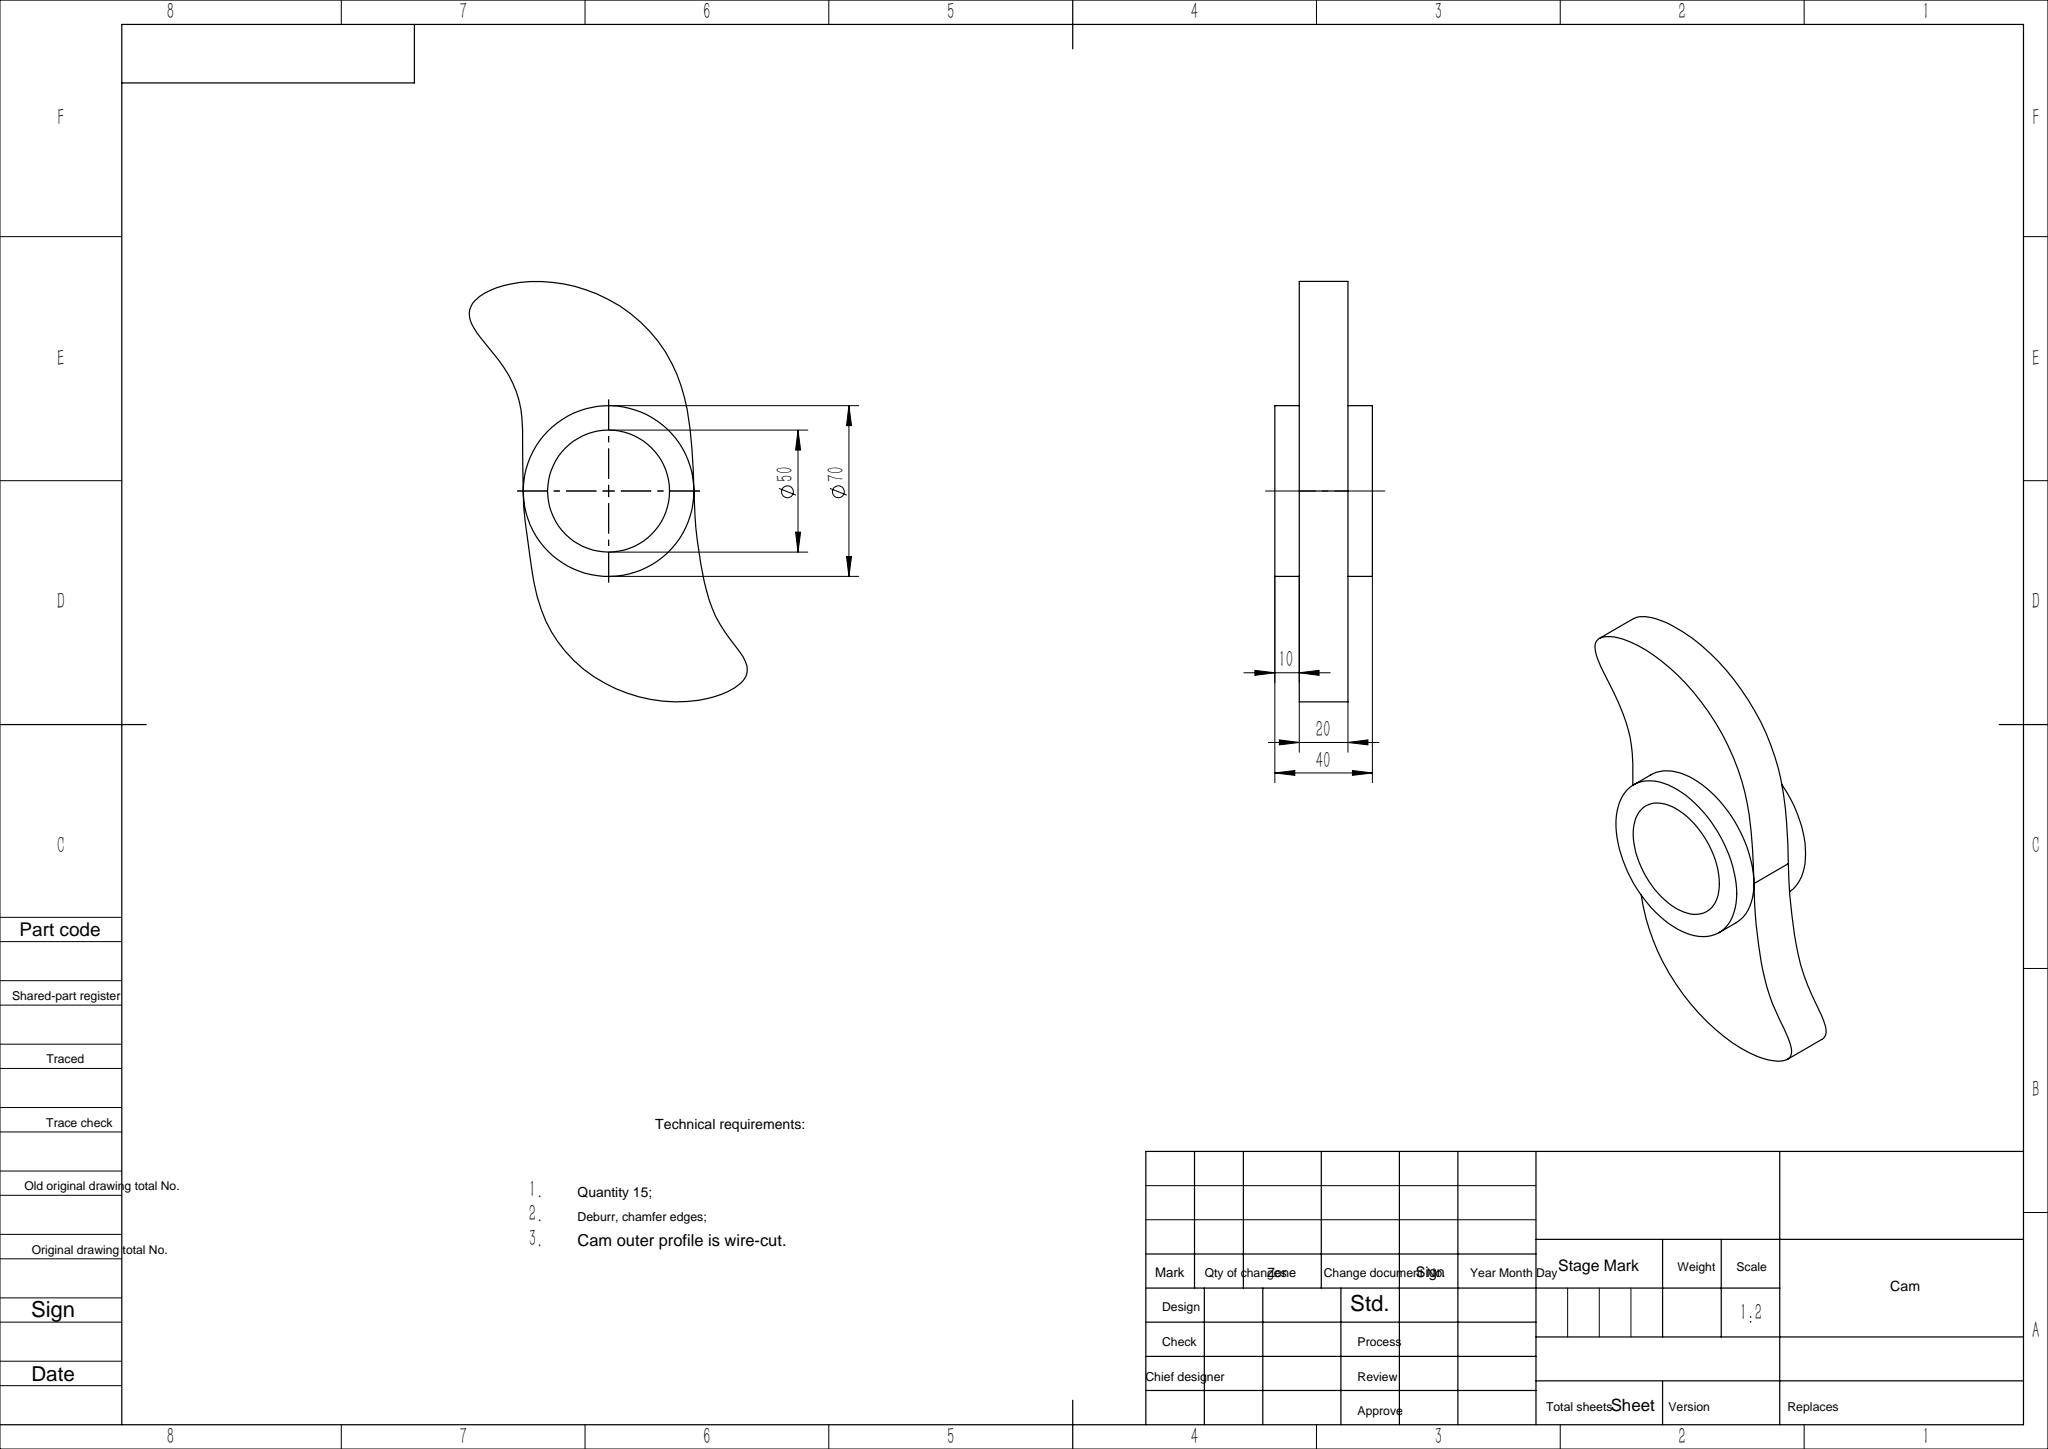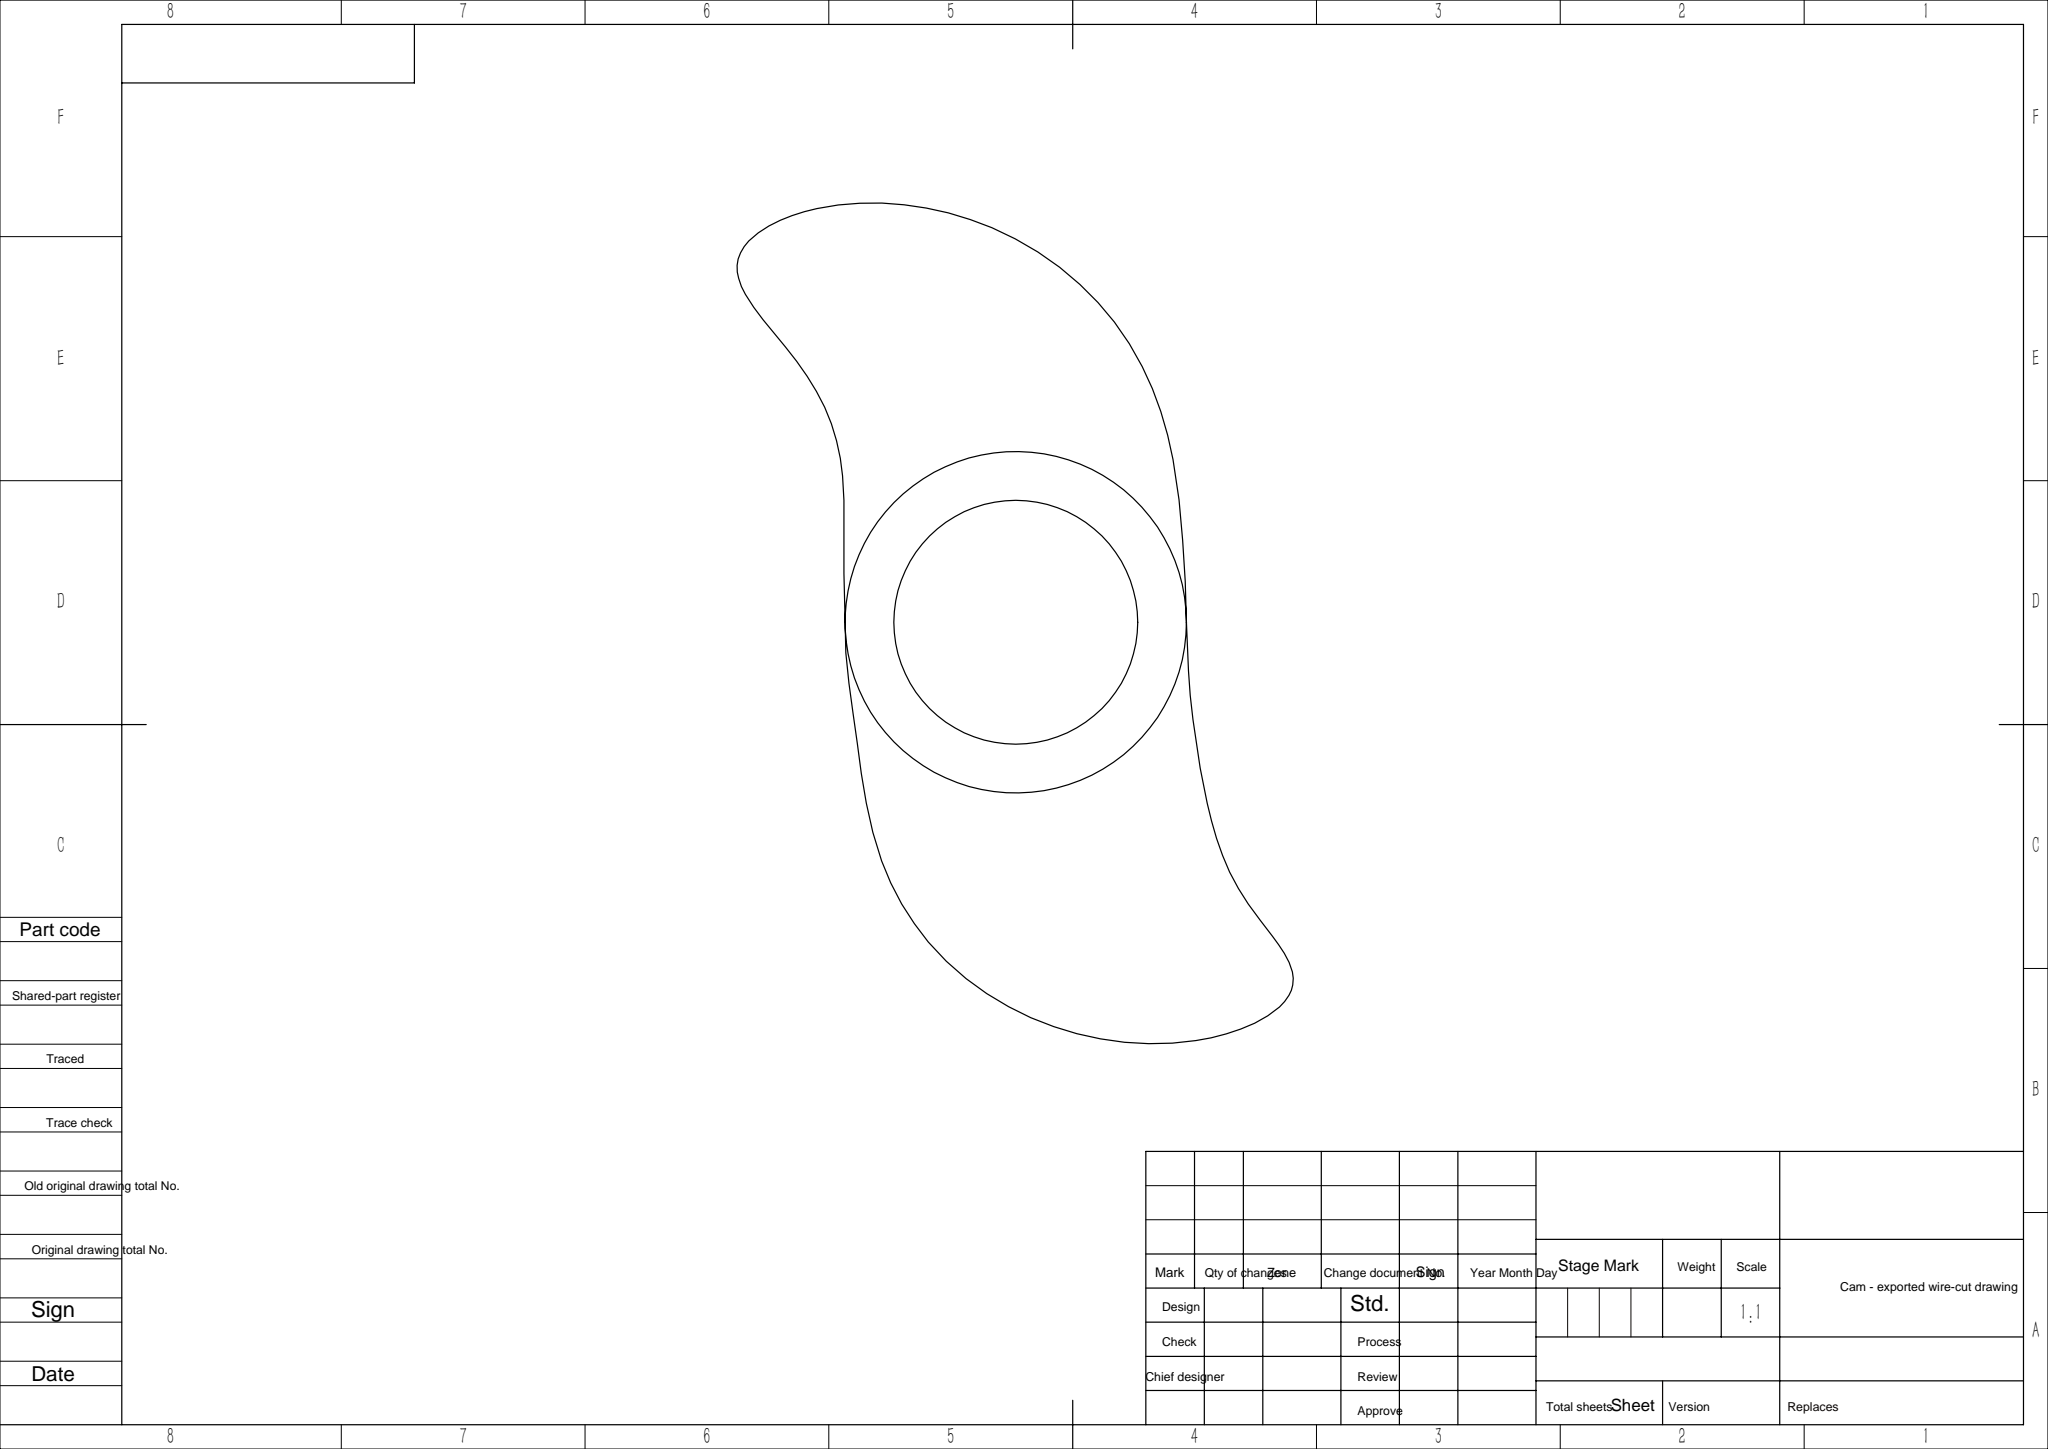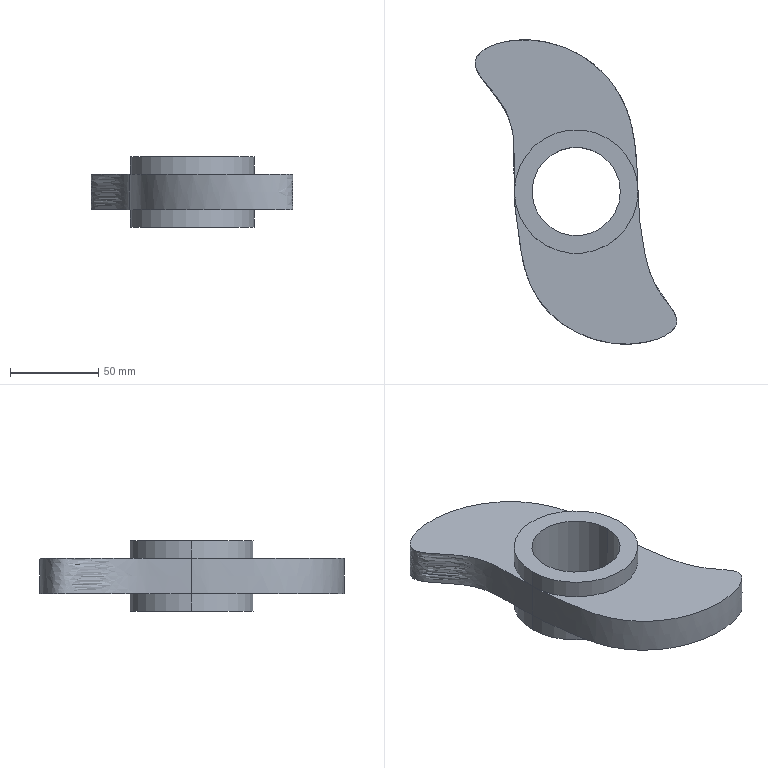Part | SolidWorks | features BaseBody 1 | 1 solid | 14 faces | box 114.053 x 172.33 x 40 mm | volume 212342 mm3 | cylinder 6 | plane 6 | spline 2 | commonest cylinder face diameters 70 x4 50 x2